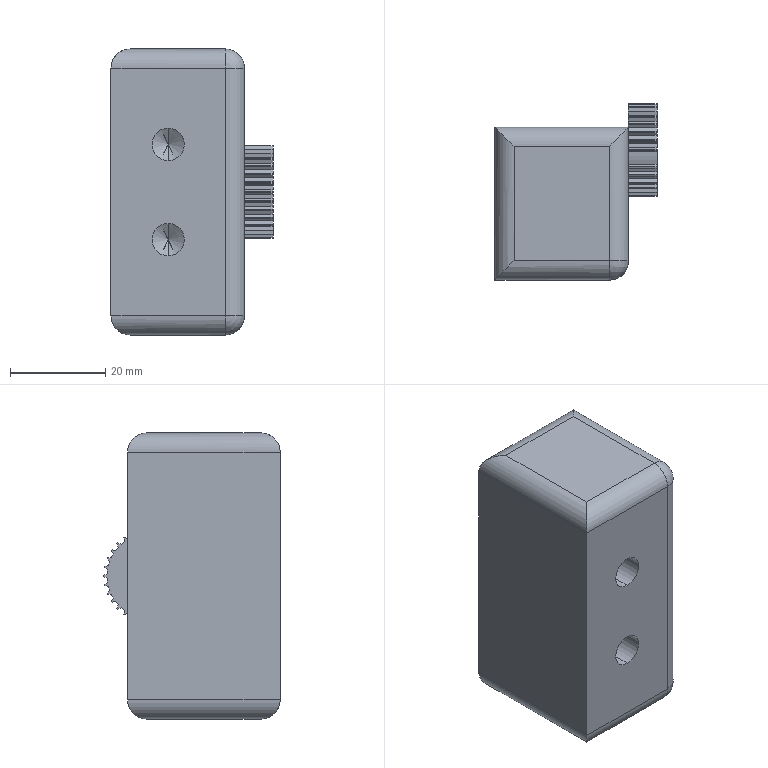Part | SolidWorks | features Extrusion 1, Fillet 1, HoleWzd 1, ICE 1 | 1 solid | 151 faces | box 34 x 36.976 x 60 mm | volume 53977 mm3 | plane 101 | cylinder 44 | cone 4 | sphere 2 | commonest cylinder face diameters 18 x31 8 x9 6.8 x4